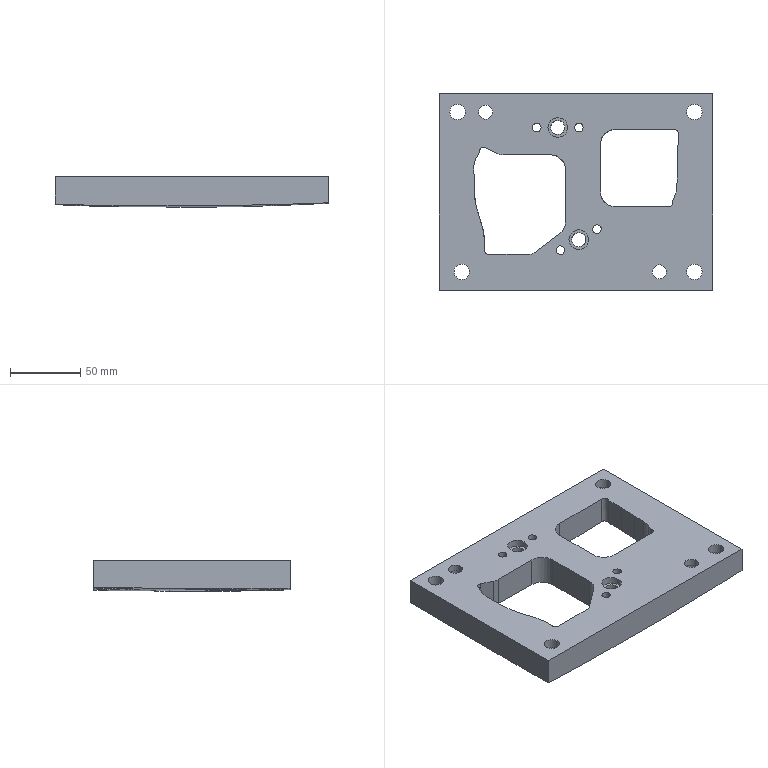Part | STEP file | 419_id2794_x_t | 1 solid | 78 faces | box 195 x 140 x 21.724 mm | volume 388406 mm3 | cylinder 34 | plane 26 | spline 18 | commonest cylinder face diameters 11 x5 4 x4 6 x4 6.1 x4 10 x4 17 x4